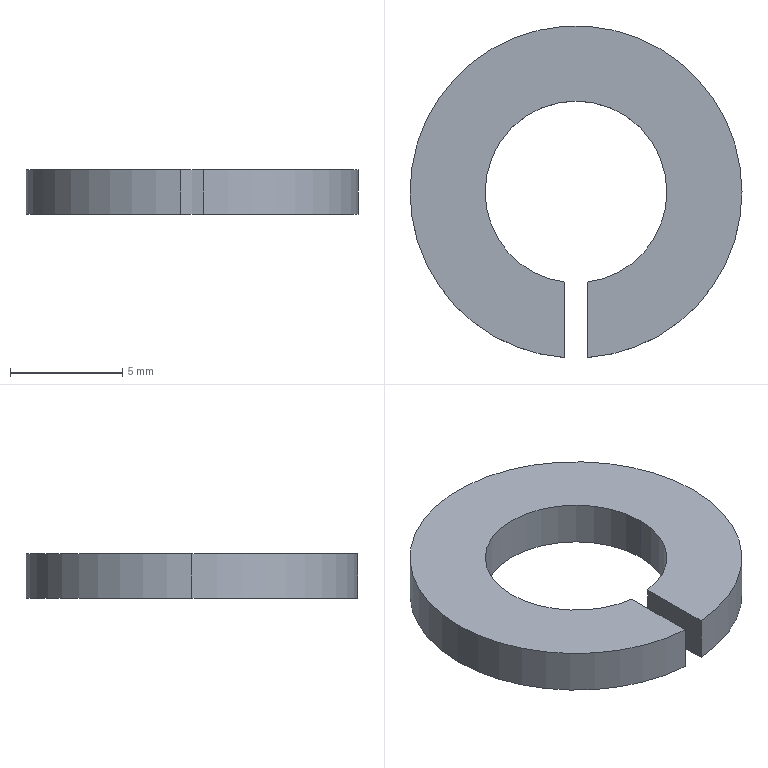Part | NX | features BREP 1 | 1 solid | 10 faces | box 14.8 x 14.783 x 2 mm | volume 234.298 mm3 | cylinder 6 | plane 4 | commonest cylinder face diameters 8.1 x3 14.8 x3
STEP:
#1=CARTESIAN_POINT('',(4.05,0.,2.));
#2=VERTEX_POINT('',#1);
#3=CARTESIAN_POINT('',(0.5,-4.019,2.));
#4=VERTEX_POINT('',#3);
#5=CARTESIAN_POINT('',(0.,0.,2.));
#6=DIRECTION('',(0.,0.,-1.));
#7=DIRECTION('',(1.,0.,0.));
#8=AXIS2_PLACEMENT_3D('',#5,#6,#7);
#9=CIRCLE('',#8,4.05);
#10=EDGE_CURVE('',#2,#4,#9,.T.);
#11=ORIENTED_EDGE('',*,*,#10,.F.);
#12=CARTESIAN_POINT('',(4.05,0.,0.));
#13=VERTEX_POINT('',#12);
#14=CARTESIAN_POINT('',(4.05,0.,2.));
#15=DIRECTION('',(0.,0.,-1.));
#16=VECTOR('',#15,1000.);
#17=LINE('',#14,#16);
#18=EDGE_CURVE('',#2,#13,#17,.T.);
#19=ORIENTED_EDGE('',*,*,#18,.T.);
#20=CARTESIAN_POINT('',(0.5,-4.019,0.));
#21=VERTEX_POINT('',#20);
#22=CARTESIAN_POINT('',(0.,0.,0.));
#23=DIRECTION('',(0.,0.,-1.));
#24=DIRECTION('',(1.,0.,0.));
#25=AXIS2_PLACEMENT_3D('',#22,#23,#24);
#26=CIRCLE('',#25,4.05);
#27=EDGE_CURVE('',#13,#21,#26,.T.);
#28=ORIENTED_EDGE('',*,*,#27,.T.);
#29=CARTESIAN_POINT('',(0.5,-4.019,2.));
#30=DIRECTION('',(0.,0.,-1.));
#31=VECTOR('',#30,1000.);
#32=LINE('',#29,#31);
#33=EDGE_CURVE('',#4,#21,#32,.T.);
#34=ORIENTED_EDGE('',*,*,#33,.F.);
#35=EDGE_LOOP('',(#11,#19,#28,#34));
#36=FACE_BOUND('',#35,.T.);
#37=CARTESIAN_POINT('',(0.,0.,2.));
#38=DIRECTION('',(0.,0.,-1.));
#39=DIRECTION('',(-1.,0.,0.));
#40=AXIS2_PLACEMENT_3D('',#37,#38,#39);
#41=CYLINDRICAL_SURFACE('',#40,4.05);
#42=ADVANCED_FACE('',(#36),#41,.F.);
#43=ORIENTED_EDGE('',*,*,#18,.F.);
#44=CARTESIAN_POINT('',(-4.05,0.,2.));
#45=VERTEX_POINT('',#44);
#46=CARTESIAN_POINT('',(0.,0.,2.));
#47=DIRECTION('',(0.,0.,-1.));
#48=DIRECTION('',(1.,0.,0.));
#49=AXIS2_PLACEMENT_3D('',#46,#47,#48);
#50=CIRCLE('',#49,4.05);
#51=EDGE_CURVE('',#45,#2,#50,.T.);
#52=ORIENTED_EDGE('',*,*,#51,.F.);
#53=CARTESIAN_POINT('',(-4.05,0.,0.));
#54=VERTEX_POINT('',#53);
#55=CARTESIAN_POINT('',(-4.05,0.,2.));
#56=DIRECTION('',(0.,0.,-1.));
#57=VECTOR('',#56,1000.);
#58=LINE('',#55,#57);
#59=EDGE_CURVE('',#45,#54,#58,.T.);
#60=ORIENTED_EDGE('',*,*,#59,.T.);
#61=CARTESIAN_POINT('',(0.,0.,0.));
#62=DIRECTION('',(0.,0.,-1.));
#63=DIRECTION('',(1.,0.,0.));
#64=AXIS2_PLACEMENT_3D('',#61,#62,#63);
#65=CIRCLE('',#64,4.05);
#66=EDGE_CURVE('',#54,#13,#65,.T.);
#67=ORIENTED_EDGE('',*,*,#66,.T.);
#68=EDGE_LOOP('',(#43,#52,#60,#67));
#69=FACE_BOUND('',#68,.T.);
#70=CARTESIAN_POINT('',(0.,0.,2.));
#71=DIRECTION('',(0.,0.,-1.));
#72=DIRECTION('',(-1.,0.,0.));
#73=AXIS2_PLACEMENT_3D('',#70,#71,#72);
#74=CYLINDRICAL_SURFACE('',#73,4.05);
#75=ADVANCED_FACE('',(#69),#74,.F.);
#76=CARTESIAN_POINT('',(7.4,0.,2.));
#77=VERTEX_POINT('',#76);
#78=CARTESIAN_POINT('',(-7.4,0.,2.));
#79=VERTEX_POINT('',#78);
#80=CARTESIAN_POINT('',(0.,0.,2.));
#81=DIRECTION('',(0.,0.,1.));
#82=DIRECTION('',(1.,0.,0.));
#83=AXIS2_PLACEMENT_3D('',#80,#81,#82);
#84=CIRCLE('',#83,7.4);
#85=EDGE_CURVE('',#77,#79,#84,.T.);
#86=ORIENTED_EDGE('',*,*,#85,.F.);
#87=CARTESIAN_POINT('',(7.4,0.,0.));
#88=VERTEX_POINT('',#87);
#89=CARTESIAN_POINT('',(7.4,0.,2.));
#90=DIRECTION('',(0.,0.,-1.));
#91=VECTOR('',#90,1000.);
#92=LINE('',#89,#91);
#93=EDGE_CURVE('',#77,#88,#92,.T.);
#94=ORIENTED_EDGE('',*,*,#93,.T.);
#95=CARTESIAN_POINT('',(-7.4,0.,0.));
#96=VERTEX_POINT('',#95);
#97=CARTESIAN_POINT('',(0.,0.,0.));
#98=DIRECTION('',(0.,0.,1.));
#99=DIRECTION('',(1.,0.,0.));
#100=AXIS2_PLACEMENT_3D('',#97,#98,#99);
#101=CIRCLE('',#100,7.4);
#102=EDGE_CURVE('',#88,#96,#101,.T.);
#103=ORIENTED_EDGE('',*,*,#102,.T.);
#104=CARTESIAN_POINT('',(-7.4,0.,2.));
#105=DIRECTION('',(0.,0.,-1.));
#106=VECTOR('',#105,1000.);
#107=LINE('',#104,#106);
#108=EDGE_CURVE('',#79,#96,#107,.T.);
#109=ORIENTED_EDGE('',*,*,#108,.F.);
#110=EDGE_LOOP('',(#86,#94,#103,#109));
#111=FACE_BOUND('',#110,.T.);
#112=CARTESIAN_POINT('',(0.,0.,2.));
#113=DIRECTION('',(0.,0.,-1.));
#114=DIRECTION('',(-1.,0.,0.));
#115=AXIS2_PLACEMENT_3D('',#112,#113,#114);
#116=CYLINDRICAL_SURFACE('',#115,7.4);
#117=ADVANCED_FACE('',(#111),#116,.T.);
#118=CARTESIAN_POINT('',(-0.5,-7.383,2.));
#119=VERTEX_POINT('',#118);
#120=CARTESIAN_POINT('',(0.,0.,2.));
#121=DIRECTION('',(0.,0.,1.));
#122=DIRECTION('',(1.,0.,0.));
#123=AXIS2_PLACEMENT_3D('',#120,#121,#122);
#124=CIRCLE('',#123,7.4);
#125=EDGE_CURVE('',#79,#119,#124,.T.);
#126=ORIENTED_EDGE('',*,*,#125,.F.);
#127=ORIENTED_EDGE('',*,*,#108,.T.);
#128=CARTESIAN_POINT('',(-0.5,-7.383,0.));
#129=VERTEX_POINT('',#128);
#130=CARTESIAN_POINT('',(0.,0.,0.));
#131=DIRECTION('',(0.,0.,1.));
#132=DIRECTION('',(1.,0.,0.));
#133=AXIS2_PLACEMENT_3D('',#130,#131,#132);
#134=CIRCLE('',#133,7.4);
#135=EDGE_CURVE('',#96,#129,#134,.T.);
#136=ORIENTED_EDGE('',*,*,#135,.T.);
#137=CARTESIAN_POINT('',(-0.5,-7.383,2.));
#138=DIRECTION('',(0.,0.,-1.));
#139=VECTOR('',#138,1000.);
#140=LINE('',#137,#139);
#141=EDGE_CURVE('',#119,#129,#140,.T.);
#142=ORIENTED_EDGE('',*,*,#141,.F.);
#143=EDGE_LOOP('',(#126,#127,#136,#142));
#144=FACE_BOUND('',#143,.T.);
#145=CARTESIAN_POINT('',(0.,0.,2.));
#146=DIRECTION('',(0.,0.,-1.));
#147=DIRECTION('',(-1.,0.,0.));
#148=AXIS2_PLACEMENT_3D('',#145,#146,#147);
#149=CYLINDRICAL_SURFACE('',#148,7.4);
#150=ADVANCED_FACE('',(#144),#149,.T.);
#151=ORIENTED_EDGE('',*,*,#93,.F.);
#152=CARTESIAN_POINT('',(0.5,-7.383,2.));
#153=VERTEX_POINT('',#152);
#154=CARTESIAN_POINT('',(0.,0.,2.));
#155=DIRECTION('',(0.,0.,1.));
#156=DIRECTION('',(1.,0.,0.));
#157=AXIS2_PLACEMENT_3D('',#154,#155,#156);
#158=CIRCLE('',#157,7.4);
#159=EDGE_CURVE('',#153,#77,#158,.T.);
#160=ORIENTED_EDGE('',*,*,#159,.F.);
#161=CARTESIAN_POINT('',(0.5,-7.383,0.));
#162=VERTEX_POINT('',#161);
#163=CARTESIAN_POINT('',(0.5,-7.383,2.));
#164=DIRECTION('',(0.,0.,-1.));
#165=VECTOR('',#164,1000.);
#166=LINE('',#163,#165);
#167=EDGE_CURVE('',#153,#162,#166,.T.);
#168=ORIENTED_EDGE('',*,*,#167,.T.);
#169=CARTESIAN_POINT('',(0.,0.,0.));
#170=DIRECTION('',(0.,0.,1.));
#171=DIRECTION('',(1.,0.,0.));
#172=AXIS2_PLACEMENT_3D('',#169,#170,#171);
#173=CIRCLE('',#172,7.4);
#174=EDGE_CURVE('',#162,#88,#173,.T.);
#175=ORIENTED_EDGE('',*,*,#174,.T.);
#176=EDGE_LOOP('',(#151,#160,#168,#175));
#177=FACE_BOUND('',#176,.T.);
#178=CARTESIAN_POINT('',(0.,0.,2.));
#179=DIRECTION('',(0.,0.,-1.));
#180=DIRECTION('',(-1.,0.,0.));
#181=AXIS2_PLACEMENT_3D('',#178,#179,#180);
#182=CYLINDRICAL_SURFACE('',#181,7.4);
#183=ADVANCED_FACE('',(#177),#182,.T.);
#184=CARTESIAN_POINT('',(-0.5,-4.019,0.));
#185=VERTEX_POINT('',#184);
#186=CARTESIAN_POINT('',(-0.5,-4.019,0.));
#187=DIRECTION('',(0.,1.,0.));
#188=VECTOR('',#187,1000.);
#189=LINE('',#186,#188);
#190=EDGE_CURVE('',#129,#185,#189,.T.);
#191=ORIENTED_EDGE('',*,*,#190,.T.);
#192=CARTESIAN_POINT('',(-0.5,-4.019,2.));
#193=VERTEX_POINT('',#192);
#194=CARTESIAN_POINT('',(-0.5,-4.019,2.));
#195=DIRECTION('',(0.,0.,-1.));
#196=VECTOR('',#195,1000.);
#197=LINE('',#194,#196);
#198=EDGE_CURVE('',#193,#185,#197,.T.);
#199=ORIENTED_EDGE('',*,*,#198,.F.);
#200=CARTESIAN_POINT('',(-0.5,-4.019,2.));
#201=DIRECTION('',(0.,1.,0.));
#202=VECTOR('',#201,1000.);
#203=LINE('',#200,#202);
#204=EDGE_CURVE('',#119,#193,#203,.T.);
#205=ORIENTED_EDGE('',*,*,#204,.F.);
#206=ORIENTED_EDGE('',*,*,#141,.T.);
#207=EDGE_LOOP('',(#191,#199,#205,#206));
#208=FACE_BOUND('',#207,.T.);
#209=CARTESIAN_POINT('',(-0.5,-4.019,2.));
#210=DIRECTION('',(-1.,0.,0.));
#211=DIRECTION('',(0.,0.,1.));
#212=AXIS2_PLACEMENT_3D('',#209,#210,#211);
#213=PLANE('',#212);
#214=ADVANCED_FACE('',(#208),#213,.F.);
#215=ORIENTED_EDGE('',*,*,#59,.F.);
#216=CARTESIAN_POINT('',(0.,0.,2.));
#217=DIRECTION('',(0.,0.,-1.));
#218=DIRECTION('',(1.,0.,0.));
#219=AXIS2_PLACEMENT_3D('',#216,#217,#218);
#220=CIRCLE('',#219,4.05);
#221=EDGE_CURVE('',#193,#45,#220,.T.);
#222=ORIENTED_EDGE('',*,*,#221,.F.);
#223=ORIENTED_EDGE('',*,*,#198,.T.);
#224=CARTESIAN_POINT('',(0.,0.,0.));
#225=DIRECTION('',(0.,0.,-1.));
#226=DIRECTION('',(1.,0.,0.));
#227=AXIS2_PLACEMENT_3D('',#224,#225,#226);
#228=CIRCLE('',#227,4.05);
#229=EDGE_CURVE('',#185,#54,#228,.T.);
#230=ORIENTED_EDGE('',*,*,#229,.T.);
#231=EDGE_LOOP('',(#215,#222,#223,#230));
#232=FACE_BOUND('',#231,.T.);
#233=CARTESIAN_POINT('',(0.,0.,2.));
#234=DIRECTION('',(0.,0.,-1.));
#235=DIRECTION('',(-1.,0.,0.));
#236=AXIS2_PLACEMENT_3D('',#233,#234,#235);
#237=CYLINDRICAL_SURFACE('',#236,4.05);
#238=ADVANCED_FACE('',(#232),#237,.F.);
#239=CARTESIAN_POINT('',(0.5,-4.019,0.));
#240=DIRECTION('',(0.,-1.,0.));
#241=VECTOR('',#240,1000.);
#242=LINE('',#239,#241);
#243=EDGE_CURVE('',#21,#162,#242,.T.);
#244=ORIENTED_EDGE('',*,*,#243,.T.);
#245=ORIENTED_EDGE('',*,*,#167,.F.);
#246=CARTESIAN_POINT('',(0.5,-4.019,2.));
#247=DIRECTION('',(0.,-1.,0.));
#248=VECTOR('',#247,1000.);
#249=LINE('',#246,#248);
#250=EDGE_CURVE('',#4,#153,#249,.T.);
#251=ORIENTED_EDGE('',*,*,#250,.F.);
#252=ORIENTED_EDGE('',*,*,#33,.T.);
#253=EDGE_LOOP('',(#244,#245,#251,#252));
#254=FACE_BOUND('',#253,.T.);
#255=CARTESIAN_POINT('',(0.5,-4.019,2.));
#256=DIRECTION('',(1.,0.,0.));
#257=DIRECTION('',(0.,1.,0.));
#258=AXIS2_PLACEMENT_3D('',#255,#256,#257);
#259=PLANE('',#258);
#260=ADVANCED_FACE('',(#254),#259,.F.);
#261=ORIENTED_EDGE('',*,*,#159,.T.);
#262=ORIENTED_EDGE('',*,*,#85,.T.);
#263=ORIENTED_EDGE('',*,*,#125,.T.);
#264=ORIENTED_EDGE('',*,*,#204,.T.);
#265=ORIENTED_EDGE('',*,*,#221,.T.);
#266=ORIENTED_EDGE('',*,*,#51,.T.);
#267=ORIENTED_EDGE('',*,*,#10,.T.);
#268=ORIENTED_EDGE('',*,*,#250,.T.);
#269=EDGE_LOOP('',(#261,#262,#263,#264,#265,#266,#267,#268));
#270=FACE_BOUND('',#269,.T.);
#271=CARTESIAN_POINT('',(0.,0.,2.));
#272=DIRECTION('',(0.,0.,1.));
#273=DIRECTION('',(1.,0.,0.));
#274=AXIS2_PLACEMENT_3D('',#271,#272,#273);
#275=PLANE('',#274);
#276=ADVANCED_FACE('',(#270),#275,.T.);
#277=ORIENTED_EDGE('',*,*,#174,.F.);
#278=ORIENTED_EDGE('',*,*,#243,.F.);
#279=ORIENTED_EDGE('',*,*,#27,.F.);
#280=ORIENTED_EDGE('',*,*,#66,.F.);
#281=ORIENTED_EDGE('',*,*,#229,.F.);
#282=ORIENTED_EDGE('',*,*,#190,.F.);
#283=ORIENTED_EDGE('',*,*,#135,.F.);
#284=ORIENTED_EDGE('',*,*,#102,.F.);
#285=EDGE_LOOP('',(#277,#278,#279,#280,#281,#282,#283,#284));
#286=FACE_BOUND('',#285,.T.);
#287=CARTESIAN_POINT('',(0.,0.,0.));
#288=DIRECTION('',(0.,0.,1.));
#289=DIRECTION('',(1.,0.,0.));
#290=AXIS2_PLACEMENT_3D('',#287,#288,#289);
#291=PLANE('',#290);
#292=ADVANCED_FACE('',(#286),#291,.F.);
#293=CLOSED_SHELL('',(#42,#75,#117,#150,#183,#214,#238,#260,#276,#292));
#294=MANIFOLD_SOLID_BREP('',#293);
#295=(LENGTH_UNIT()NAMED_UNIT(*)SI_UNIT(.MILLI.,.METRE.));
#296=UNCERTAINTY_MEASURE_WITH_UNIT(LENGTH_MEASURE(0.00001),#295,'','');
#297=(NAMED_UNIT(*)PLANE_ANGLE_UNIT()SI_UNIT($,.RADIAN.));
#298=(NAMED_UNIT(*)SI_UNIT($,.STERADIAN.)SOLID_ANGLE_UNIT());
#299=(GEOMETRIC_REPRESENTATION_CONTEXT(3)GLOBAL_UNCERTAINTY_ASSIGNED_CONTEXT((#296))GLOBAL_UNIT_ASSIGNED_CONTEXT((#295,#297,#298))REPRESENTATION_CONTEXT('',''));
#300=ADVANCED_BREP_SHAPE_REPRESENTATION('',(#294),#299);